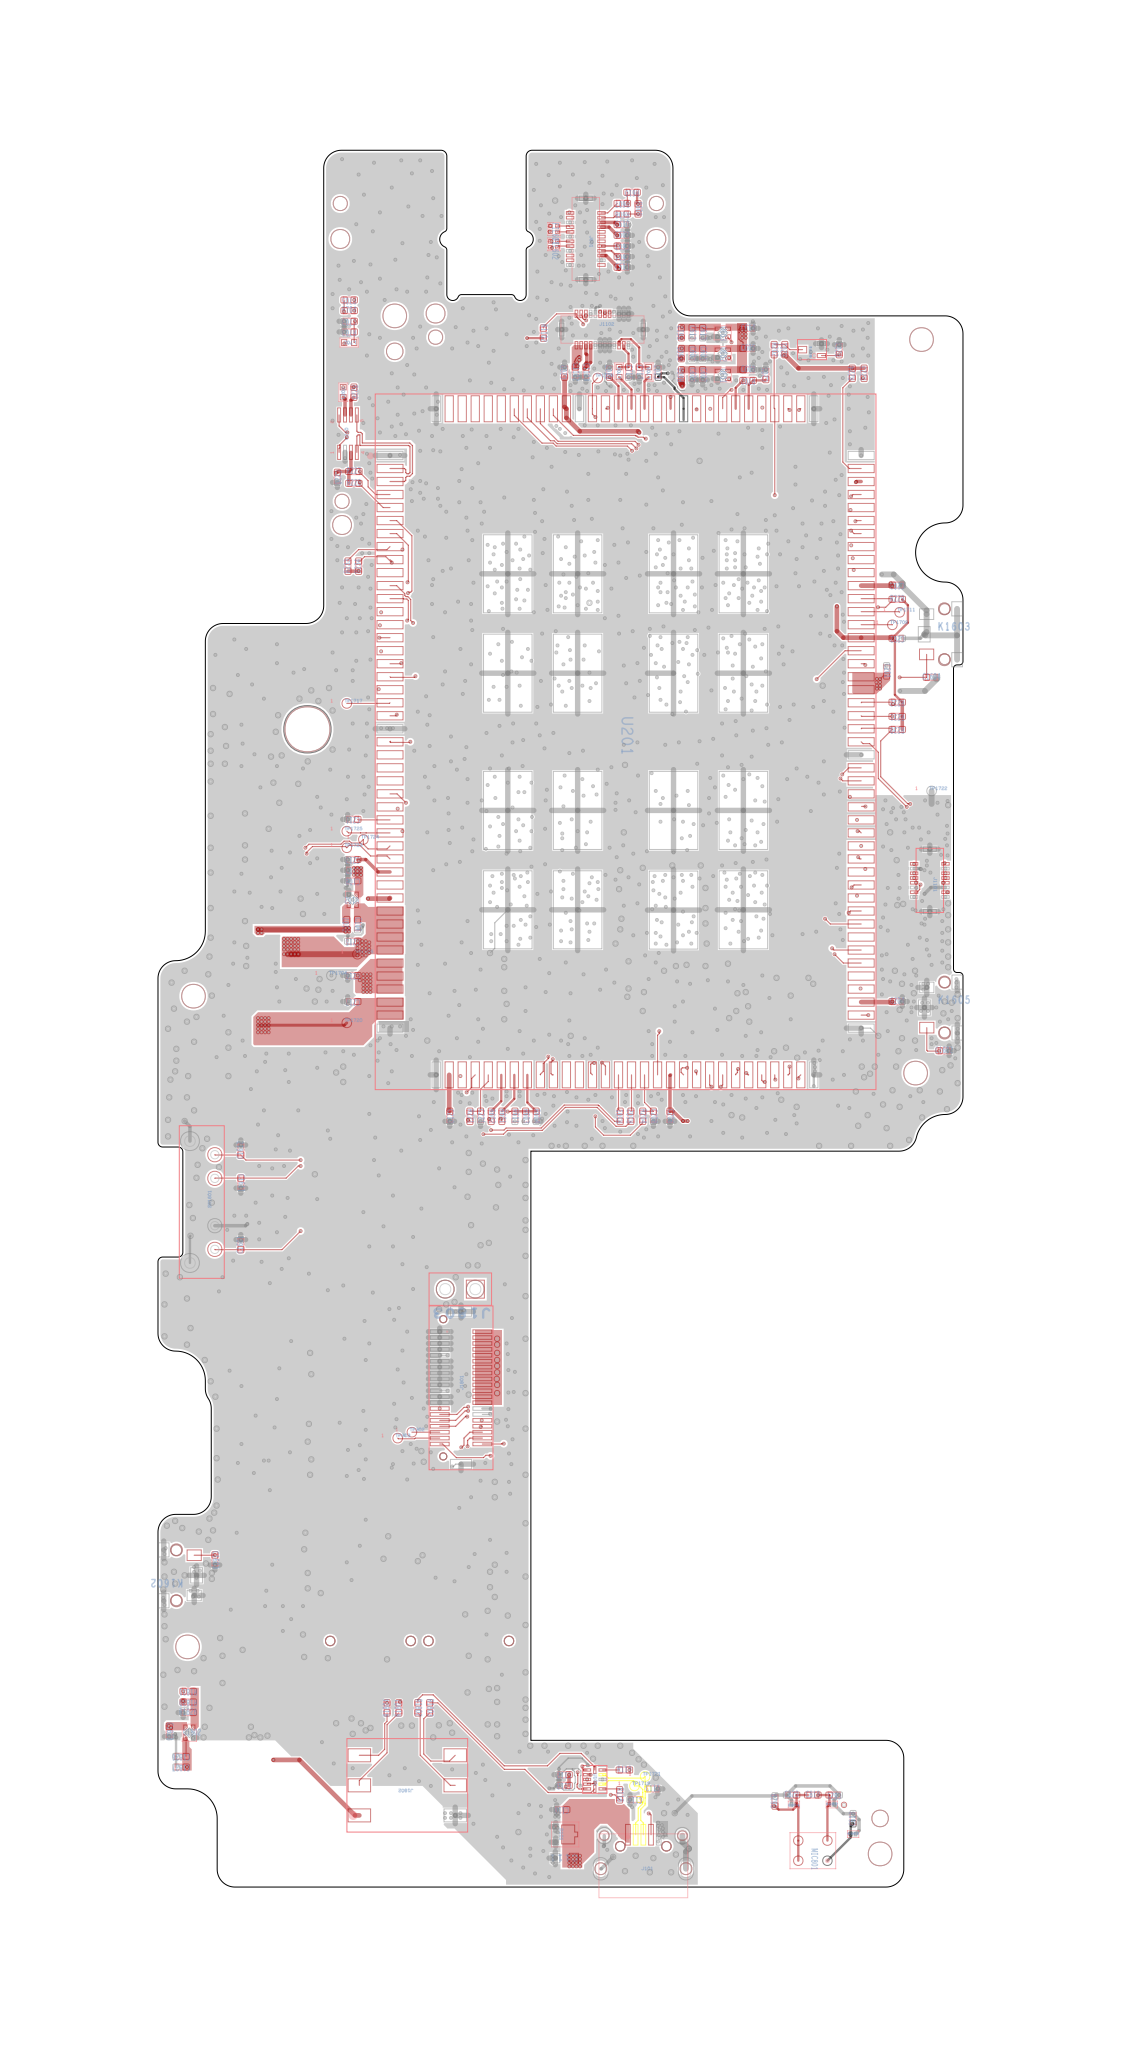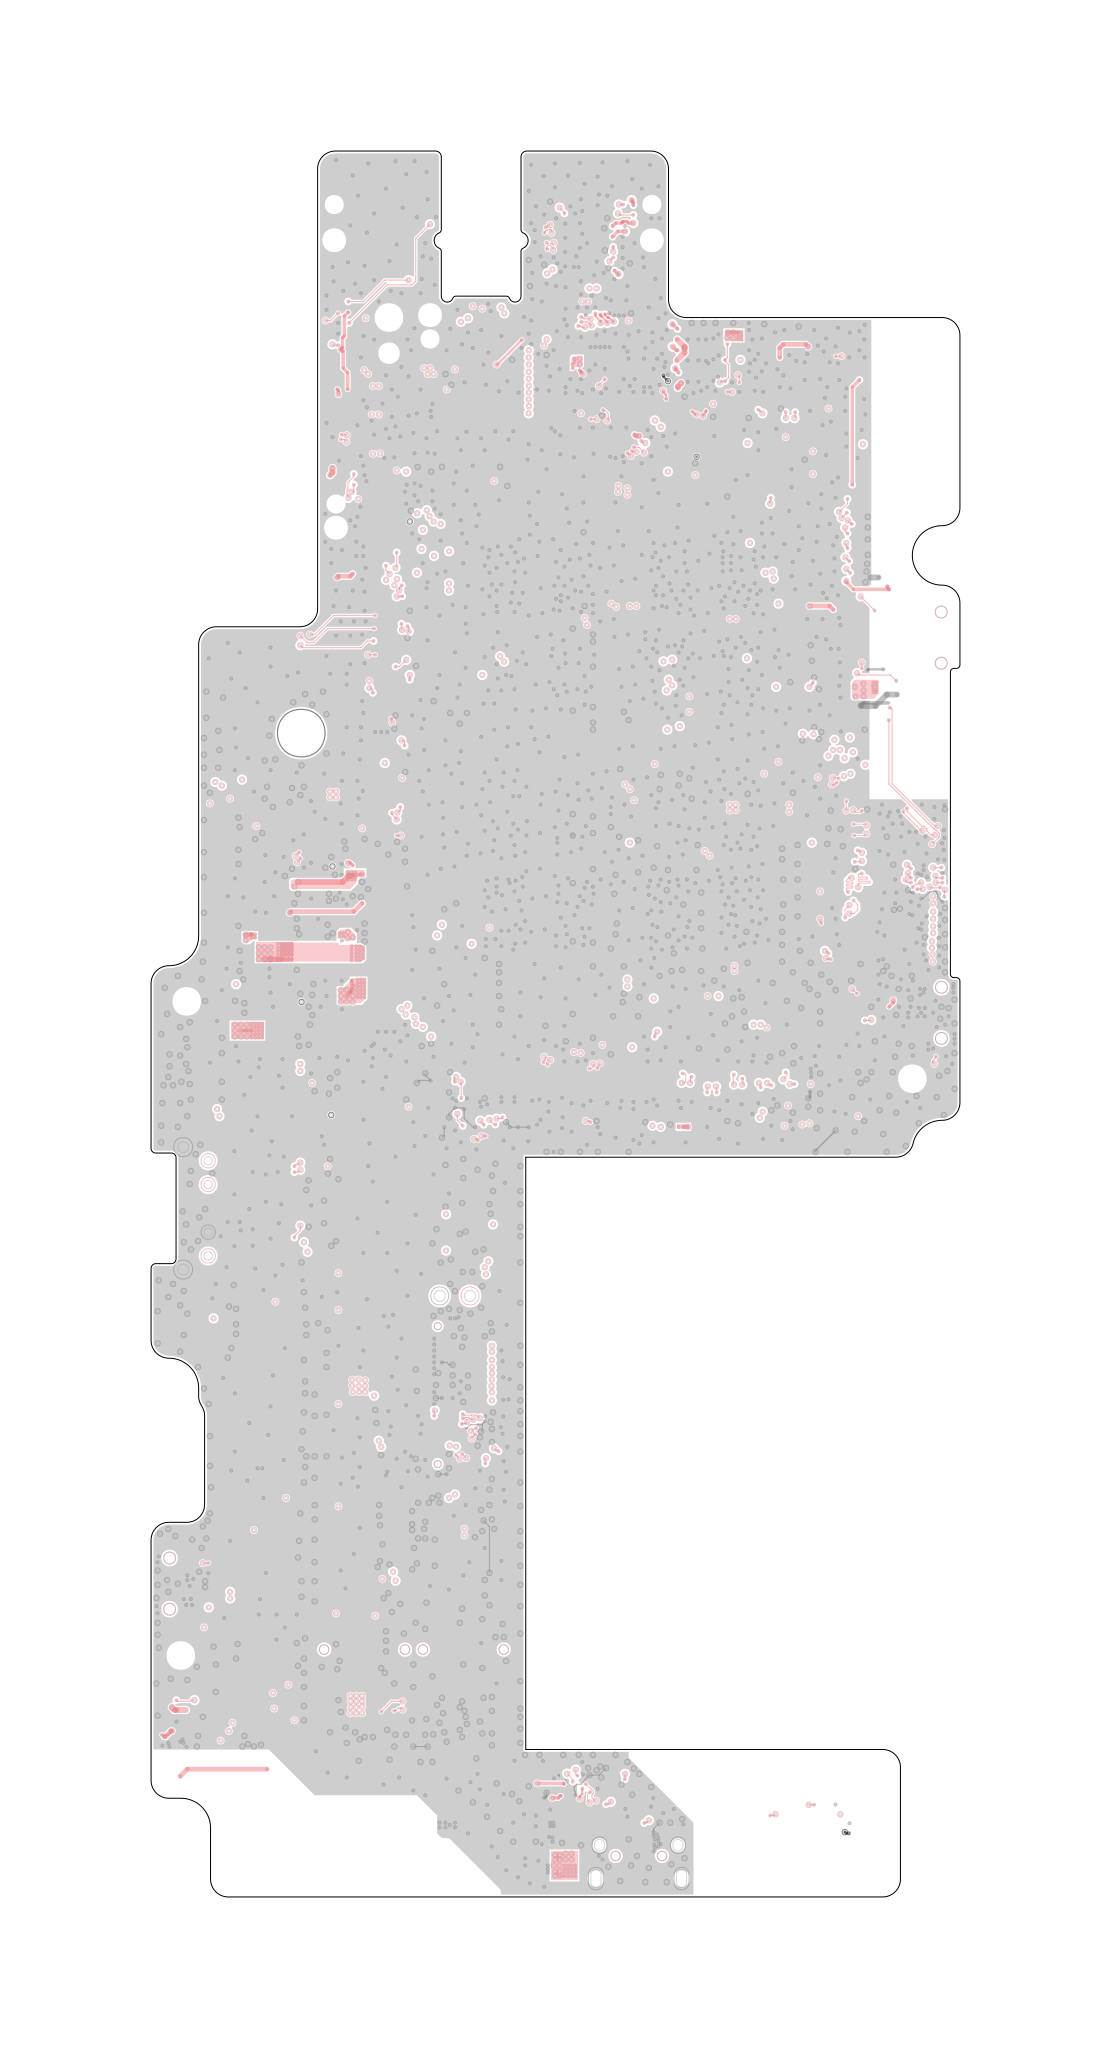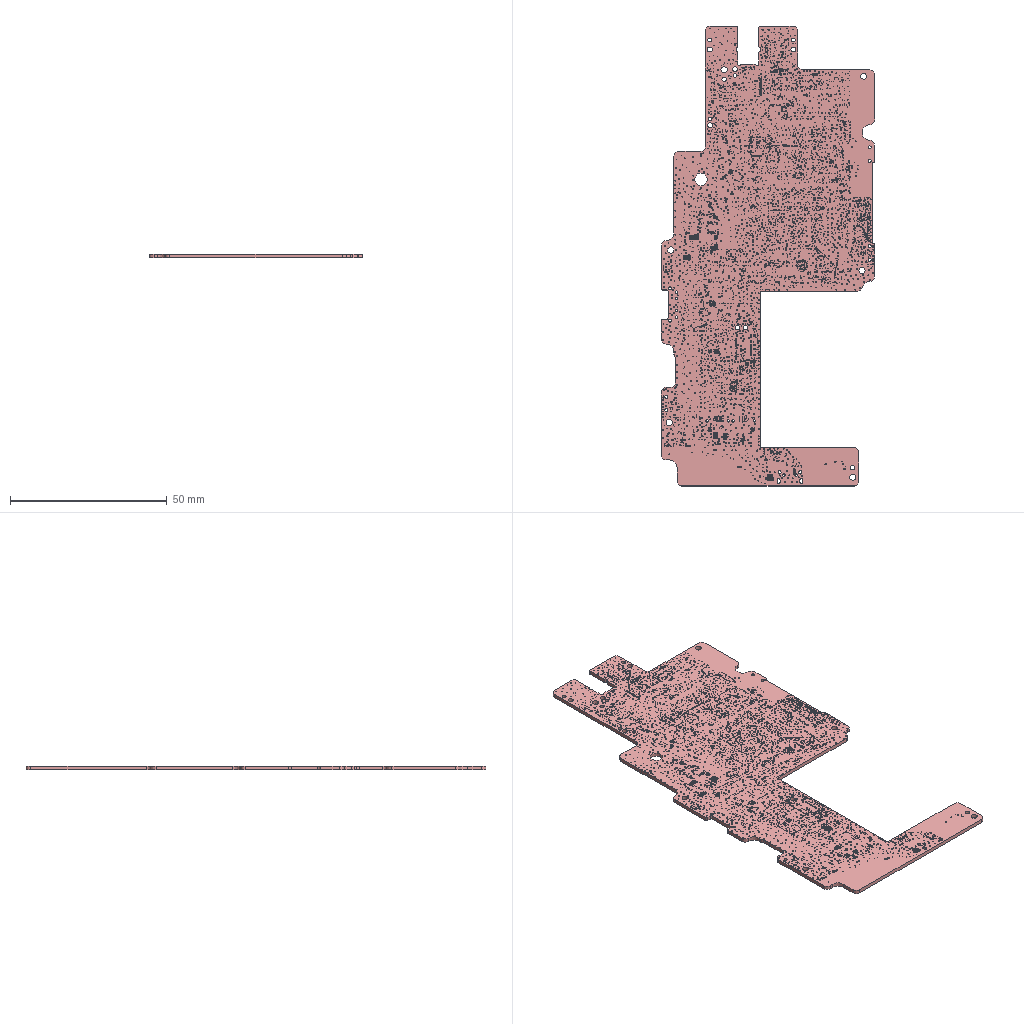Circuit board layout | Cadence Allegro | box 68 x 146.8 x 1.2 mm
Layer stack:
# Cadence Allegro layer stack of  (unit mm; from the constraint file cross-section; dielectric type: 0 not recorded (Allegro does not mark core vs prepreg), 3 surface material)
index,name,kind,layer,copper_thickness_mm,dielectric_type,dielectric_thickness_mm,dielectric_material,dielectric_constant
0,Top Surface,other,,,,,,
1,TOP,copper,TOP,0.0229,,,,
2,Dielectric1,dielectric,,,0,0.381,FR-4,4.5
3,ART02,copper,ART02,0.0178,,,,
4,Dielectric2,dielectric,,,0,0.0889,FR-4,4.5
5,ART03,copper,ART03,0.033,,,,
6,Dielectric3,dielectric,,,0,0.2032,FR-4,4.5
7,ART04,copper,ART04,0.033,,,,
8,Dielectric4,dielectric,,,0,0.0889,FR-4,4.5
9,ART05,copper,ART05,0.0178,,,,
10,Dielectric5,dielectric,,,0,0.381,FR-4,4.5
11,BOTTOM,copper,BOTTOM,0.0229,,,,
12,Bottom Surface,other,,,,,,
# drill layer pairs: low layer,high layer
drill_pair,TOP,BOTTOM
drill_pair,ART05,BOTTOM
Part placement:
REFDES,COMP_VALUE,SYM_NAME,SYM_X,SYM_Y,SYM_ROTATE,SYM_MIRROR
ANT401,BXJ-TH-164-01-W,PAD_ANT_BXJ-TH-164-01-W,147.35,169.01,90.000,YES
ANT402,BXJ-TH-164-01-W,PAD_ANT_BXJ-TH-164-01-W,144.25,169.01,90.000,YES
ANT403,BXJ-TH-164-01-W,PAD_ANT_BXJ-TH-164-01-W,157.89,263.55,180.000,YES
ANT404,BXJ-TH-164-01-W,PAD_ANT_BXJ-TH-164-01-W,157.89,260.45,180.000,YES
ANT405,BXJ-TH-164-01-W,PAD_ANT_BXJ-TH-164-01-W,150.45,169,90.000,YES
ANT406,BXJ-TH-164-01-W,PAD_ANT_BXJ-TH-164-01-W,157.9,266.65,180.000,YES
C101,22U,C0805,118.8,179.8,180.000,YES
C102,10P,C0402,117.9,190.6,270.000,YES
C104,10P,C0402,114.5,190.6,270.000,YES
C105,22U,C0805,113.4,179.8,0.000,YES
C106,1U,C0402,110.9,246.4,270.000,NO
C107,1U,C0402,110.5,251,180.000,NO
C108,10P,C0402,110.5,250.1,180.000,NO
C110,10P,C0402,128.15,171.6,180.000,NO
C111,4.7U,C0603,128.4,167.5,180.000,NO
C112,0.1U,C0402,128.35,174.55,180.000,NO
C113,1U,C0402,128.35,173.65,180.000,NO
C114,10P,C0402,134.35,172.45,180.000,NO
C115,10P,C0402,135.85,173.35,0.000,NO
C201,1U,C0402,155.6,267.85,270.000,NO
C202,1U,C0402,156.5,270.6,180.000,NO
C203,1U,C0402,156.5,275.1,180.000,NO
C204,0.1U,C0402,156.5,239.9,0.000,NO
C205,0.1U,C0402,145.4,292.9,90.000,NO
C206,1U,C0402,137.3,230.2,270.000,NO
C207,0.1U,C0402,136.3,293.1,90.000,NO
C208,10P,C0402,135.9,230.2,270.000,NO
C209,0.1U,C0402,128.4,293.1,90.000,NO
C210,1U,C0402,118.7,230.2,270.000,NO
C211,0.1U,C0402,110.5,255.3,180.000,NO
C213,1U,C0402,110.5,251.9,180.000,NO
C215,2.2U,C0402,110.5,245,180.000,NO
C216,0.1U,C0402,110.5,242.1,180.000,NO
C217,0.1U,C0402,110.5,239.9,180.000,NO
C220,0.1U,C0402,109.2,284.2,270.000,NO
C221,10P,C0402,121.3,230.2,270.000,NO
C224,1U,C0402,146.2,272.5,270.000,YES
C225,10P,C0402,147.1,272.5,270.000,YES
C226,1U,C0402,142.4,272.9,0.000,YES
C227,0.1U,C0402,148.9,272.5,270.000,YES
C301,0.1U,C0402,114.8,223.3,180.000,YES
C302,0.1U,C0402,114.8,228.1,0.000,YES
C303,1U,C0402,106.2,228,90.000,YES
C304,1U,C0402,105,224.7,270.000,YES
C305,0.1U,C0402,105.9,224.7,270.000,YES
C306,1U,C0402,116.1,217.7,0.000,YES
C307,1U,C0402,114,219.65,0.000,YES
C308,10P,C0402,114.45,218.3,90.000,YES
C309,0.1U,C0402,108.9,218.3,90.000,YES
C310,0.1U,C0402,105.9,222.9,90.000,YES
C401,10P,C0402,158.6,289,90.000,YES
C402,0.1U,C0402,124.2,286.7,180.000,YES
C403,470P,C0402,125.7,271.6,90.000,YES
C404,4.7U,C0603,121.9,286.8,0.000,YES
C405,100P,C0402,119.8,272.6,0.000,YES
C406,0.1U,C0402,119.8,271.7,0.000,YES
C407,1U,C0402,112.9,286,90.000,YES
C408,10P,C0402,113.8,286,90.000,YES
C409,1U,C0402,109.5,286,90.000,YES
C410,1U,C0402,110.3,284.6,0.000,YES
C411,0.1U,C0402,119.5,286.7,0.000,YES
C501,1U,C0402,114.4,291.1,90.000,YES
C502,10P,C0402,115.3,291.1,90.000,YES
C503,1U,C0402,110.4,291.6,0.000,YES
C504,1U,C0402,114.4,293,90.000,YES
C505,10P,C0402,115.3,293,90.000,YES
C506,1U,C0402,110.4,293.5,0.000,YES
C507,0.1U,C0402,117.046,261.786,180.000,YES
C508,4.7U,C0402,117.046,262.687,180.000,YES
C509,10U,C0603,114.2,267.7,0.000,YES
C510,10P,C0402,116.1,268.4,270.000,YES
C511,1U,C0402,110.4,289.7,0.000,YES
C512,1U,C0402,115.3,289.2,90.000,YES
C513,10P,C0402,114.4,289.2,90.000,YES
C520,10P,C0402,122.5,298,0.000,YES
C521,10P,C0402,120.7,298,180.000,YES
C522,1U,C0402,117.7,286.7,180.000,YES
C523,10P,C0402,115.9,286.7,0.000,YES
C524,0.1U,C0402,116.2,293,90.000,YES
C525,0.1U,C0402,116.6,290.7,0.000,YES
C526,0.1U,C0402,117.1,289.2,90.000,YES
C601,1U,C0402,140.062,294.669,270.000,NO
C602,10P,C0402,139.162,294.669,270.000,NO
C603,10P,C0402,133.273,303.763,180.000,NO
C604,10P,C0402,133.273,302.863,180.000,NO
C605,1U,C0402,143.9,295.1,0.000,NO
C606,1U,C0402,139.162,292.869,270.000,NO
C607,10P,C0402,140.062,292.869,270.000,NO
C608,1U,C0402,143.9,293.3,0.000,NO
C609,0.1U,C0402,133.273,304.663,0.000,NO
C610,0.1U,C0402,133.273,305.563,0.000,NO
C611,0.1U,C0402,133.273,301.963,0.000,NO
C612,1U,C0402,139.162,296.431,270.000,NO
C613,10P,C0402,140.062,296.431,270.000,NO
C614,1U,C0402,143.9,296.8,0.000,NO
C701,220N,C0402,137.4,268.7,0.000,YES
C702,33P,C0402,109.1,298.8,270.000,YES
C703,33P,C0402,110.2,297.4,180.000,NO
C704,33P,C0402,133.2,296.5,180.000,YES
C705,1U,C0402,133.2,297.4,0.000,YES
C706,33P,C0402,113.5,299.5,180.000,YES
C707,0.1U,C0402,126.7,249.9,0.000,YES
C708,1U,C0402,127.1,255.1,270.000,YES
C709,10P,C0402,128,255.1,270.000,YES
C710,1U,C0402,131.4,255,270.000,YES
C711,22U,C0805,131.2,251.1,90.000,YES
C712,22U,C0805,129.3,251.1,90.000,YES
C713,4.7U,C0402,137.4,269.6,180.000,YES
C714,33P,C0402,134.7,293.1,270.000,NO
C715,33P,C0402,133.8,293.1,270.000,NO
C716,220N,C0402,132,268.2,180.000,YES
C717,0.1U,C0402,128.727,247.493,0.000,YES
C718,22U,C0805,131.135,244.786,270.000,YES
C719,22U,C0805,129.173,244.786,270.000,YES
C801,33N,C0402,140.8,229.4,270.000,YES
C802,0.1U,C0402,128.5,238.2,90.000,YES
C803,0.1U,C0402,139,240.9,180.000,YES
C805,33N,C0402,144.6,230,180.000,YES
C806,33N,C0402,144.6,231.8,0.000,YES
C807,220N,C0402,132.7,232.3,0.000,YES
C808,220N,C0402,129.5,232.8,270.000,YES
C809,220N,C0402,132.7,233.3,0.000,YES
C810,220N,C0402,129.5,234.7,90.000,YES
C811,220N,C0402,132.7,234.2,0.000,YES
C812,220N,C0402,133.2,236.1,270.000,YES
C813,33P,C0402,130.9,236.1,180.000,YES
C814,0.1U,C0402,129.5,237.4,90.000,YES
C817,33N,C0402,137.6,229,0.000,YES
C818,0.1U,C0402,152.77,170.83,90.000,NO
C819,33P,C0402,149.37,172.83,0.000,NO
C820,33P,C0402,147.57,172.83,0.000,NO
C821,33P,C0402,151.17,172.83,180.000,NO
C1001,1U,C0603,151.5,246,0.000,YES
C1002,33P,C0402,153.8,247.7,0.000,YES
C1003,0.1U,C0402,153.8,250.3,0.000,YES
C1004,1U,C0402,154.3,236.1,180.000,YES
C1005,33P,C0402,158,237.8,180.000,YES
C1006,33P,C0402,153.8,246.5,0.000,YES
C1007,33P,C0402,153.8,244.9,0.000,YES
C1008,33P,C0402,152,248.3,0.000,YES
C1009,0.1U,C0402,153.8,248.9,0.000,YES
C1010,0.1U,C0402,155.17,255.04,270.000,YES
C1011,1U,C0402,155.17,253.24,90.000,YES
C1101,33P,C0402,117,272.1,90.000,YES
C1102,0.1U,C0402,129.3,293.1,270.000,NO
C1103,0.1U,C0402,130.2,293.1,270.000,NO
C1104,0.1U,C0402,109.3,277.4,0.000,YES
C1105,33P,C0402,116.1,272.1,270.000,YES
C1106,33P,C0402,113.1,278,0.000,YES
C1107,1U,C0402,100.7,182,0.000,YES
C1201,1UF,C0402,126.5,263.7,90.000,YES
C1202,0.1U,C0402,98,187.3,90.000,YES
C1203,1U,C0402,99.3,187.3,90.000,YES
C1204,0.1U,C0402,101.4,187.3,90.000,YES
C1205,1U,C0402,100.2,187.3,90.000,YES
C1206,0.1U,C0402,136.9,266.9,180.000,YES
C1207,1U,C0402,135.1,266.9,0.000,YES
C1208,0.1U,C0402,132.8,262.8,0.000,YES
C1209,0.1U,C0402,132.8,264.6,0.000,YES
C1501,10P,C0402,111,238.7,270.000,YES
C1502,1U,C0402,116.2,237.4,0.000,YES
C1503,33P,C0402,116.2,238.3,180.000,YES
C1504,10P,C0402,111.9,238.7,270.000,YES
C1505,10P,C0402,114.8,238.7,270.000,YES
C1506,10P,C0402,117.6,238.7,90.000,YES
C1507,10P,C0402,120.4,238.7,270.000,YES
C1508,10P,C0402,121.3,238.7,270.000,YES
C1509,10P,C0402,143.2,258,0.000,YES
C1510,10P,C0402,135.4,258,0.000,YES
C1511,10P,C0402,138,258,0.000,YES
C1512,10P,C0402,140.6,258,0.000,YES
C1513,1U,C0402,140.6,258.9,0.000,YES
C1514,1U,C0402,147.2,258.4,270.000,YES
C1601,10P,C0402,101.049,219.352,90.000,NO
C1602,10P,C0402,160.46,235.74,0.000,NO
C1603,10P,C0402,98.86,192.7,270.000,NO
C1604,10P,C0402,159.39,267.3,0.000,NO
C1605,10P,C0402,100.7,177.9,180.000,YES
C1606,10P,C0402,100.7,178.8,180.000,YES
C1607,10P,C0402,100.7,179.7,180.000,YES
C1608,10P,C0402,105.4,233.8,180.000,YES
C1609,10P,C0402,105.4,234.7,180.000,YES
C1610,10P,C0402,105.4,235.6,180.000,YES
C1611,10P,C0402,101.049,224.552,270.000,NO
C1612,10P,C0402,101.049,227.352,90.000,NO
C1802,22U,C0805,123.7,205.8,90.000,YES
C1803,22U,C0805,123.7,212.2,270.000,YES
C1804,1U,C0402,123.7,210,180.000,YES
C1805,0.1U,C0402,123.7,209,180.000,YES
C1806,0.1U,C0402,123.7,208,180.000,YES
C1812,10U,C0603,115.2,211,270.000,YES
C1813,10U,C0603,115.2,207,90.000,YES
C1814,0.1U,C0402,112.8,199.8,180.000,YES
C1815,0.1U,C0402,121.7,193.5,0.000,YES
C1816,0.1U,C0402,123.1,202.5,180.000,YES
C1817,1U,C0402,117.8,193,0.000,YES
C1818,0.1U,C0402,112.8,198.9,0.000,YES
C1819,0.1U,C0402,121.7,195.3,180.000,YES
C1820,0.1U,C0402,108.4,198.6,180.000,YES
C1821,1U,C0402,110.3,195.5,90.000,YES
C1822,1U,C0402,112.8,198,0.000,YES
C1823,10P,C0402,112.8,197.1,0.000,YES
C1826,10P,C0402,96,176.1,180.000,NO
C1827,1U,C0402,96,175.2,180.000,NO
C1828,1U,C0402,95,178.2,270.000,NO
C1829,10P,C0402,113.5,213.7,180.000,YES
C1830,1U,C0402,113.5,214.6,180.000,YES
C1831,1U,C0402,110.3,215.4,0.000,YES
D101,PTVS12VU1UPA,DFN2020-3,128.45,169.5,270.000,NO
D801,PESD5V0L1BSF,DSN0603-2,147.77,172.03,0.000,NO
D802,PESD5V0L1BSF,DSN0603-2,150.97,172.03,180.000,NO
D803,PESD5V0L1BSF,DSN0603-2,152.77,169.53,180.000,NO
D1001,RB160MM-40,RB160MM-40,151.4,241.6,270.000,YES
D1101,PESD5V0L1BSF,DSN0603-2,112.7,277.2,0.000,YES
D1102,PESD5V0L1BSF,DSN0603-2,110.7,277.2,0.000,YES
D1103,PESD5V0L1BSF,DSN0603-2,111.7,277.2,180.000,YES
D1501,PESD5V0L1BSF,DSN0603-2,117.3,240.6,0.000,YES
D1502,PESD5V0L1BSF,DSN0603-2,116,240.6,0.000,YES
D1504,PESD5V0L1BSF,DSN0603-2,120,240.6,180.000,YES
D1505,PESD5V0L1BSF,DSN0603-2,118.6,240.6,0.000,YES
D1506,PESD5V0L1BSF,DSN0603-2,114.7,240.6,0.000,YES
D1507,PESD5V0L1BSF,DSN0603-2,113.4,240.6,180.000,YES
D1508,PESD5V0L1BSF,DSN0603-2,111.9,240.6,0.000,YES
D1509,PESD5V0L1BSF,DSN0603-2,144.5,258.2,90.000,YES
D1510,PESD5V0L1BSF,DSN0603-2,136.7,258.2,90.000,YES
D1511,PESD5V0L1BSF,DSN0603-2,139.3,258.2,90.000,YES
D1512,PESD5V0L1BSF,DSN0603-2,141.9,258.2,90.000,YES
F401,MGMA5220H2450-A01,MGMA5220H2450-A01,159,283.8,90.000,YES
F405,SAFEB1G57KB0F00,SAFEA1G57KJ0F00,123.45,272.4,180.000,YES
FIL501,ACFT4A2G900E,EMI4_0P85X0P65X0P55_INNOCHIPS,125.15,294.858,90.000,YES
FIL502,ACFT4A2G900E,EMI4_0P85X0P65X0P55_INNOCHIPS,125.15,293.658,90.000,YES
FIL503,ACFT4A2G900E,EMI4_0P85X0P65X0P55_INNOCHIPS,125.15,292.458,90.000,YES
FIL504,ACFT4A2G900E,EMI4_0P85X0P65X0P55_INNOCHIPS,125.15,291.308,90.000,YES
FIL505,ACFT4A2G900E,EMI4_0P85X0P65X0P55_INNOCHIPS,125.15,290.158,90.000,YES
FIL601,ACFT4A2G900E,EMI4_0P85X0P65X0P55_INNOCHIPS,127.5,305.2,270.000,NO
FIL602,ACFT4A2G900E,EMI4_0P85X0P65X0P55_INNOCHIPS,127.5,303.9,270.000,NO
FIL1001,ACFT4A2G900E,EMI4_0P85X0P65X0P55_INNOCHIPS,159.9,245.3,90.000,YES
FIL1002,ACFT4A2G900E,EMI4_0P85X0P65X0P55_INNOCHIPS,159.9,247.7,90.000,YES
FIL1003,ACFT4A2G900E,EMI4_0P85X0P65X0P55_INNOCHIPS,159.9,246.5,90.000,YES
FIL1004,ACFT4A2G900E,EMI4_0P85X0P65X0P55_INNOCHIPS,159.9,248.9,90.000,YES
FIL1005,ACFT4A2G900E,EMI4_0P85X0P65X0P55_INNOCHIPS,159.9,244.1,90.000,YES
J101,U1014-2-DN-W,USB_U1014-2-DN-W,135.05,166.6,0.000,NO
J102,02250370010168,CON_BAT_02250370010168,112.001,186.503,180.000,YES
J103,02250370010168,CON_BAT_02250370010168,120.301,186.503,180.000,YES
J401,20449-001E,ANT_CON_IPEX_20449-001E,128.1,275.7,0.000,YES
J402,20449-001E,ANT_CON_IPEX_20449-001E,128.05,175.52,0.000,YES
J403,20449-001E,ANT_CON_IPEX_20449-001E,159.5,291.8,0.000,YES
J406,20449-001E,ANT_CON_IPEX_20449-001E,157,273.9,0.000,YES
J601,DF37NB-24DS-0_4V,BTB_DF37NB-24DS-0_4V_CW,130.189,304.355,270.000,NO
J701,J303-B06G1-NZL2,JACK_J303-B06G1-NZL2,118.45,311.15,180.000,YES
J1001,DF37NB-24DS-0_4V,BTB_DF37NB-24DS-0_4V_CCW,157.075,246.9,270.000,YES
J1002,DF37NB-10DS-0_4V,BTB_DF37NB-10DS-0_4V_CW,158.07,254.74,270.000,YES
J1101,DF37NB-16DS-0_4V,BTB_DF37NB-16DS-0_4V_CW,159.25,250.14,270.000,NO
J1102,DF37NB-24DS-0_4V,BTB_DF37NB-24DS-0_4V_CW,131.6,296.7,0.000,NO
J1103,DF37NB-16DS-0_4V,BTB_DF37NB-16DS-0_4V_CW,111.4,274.6,0.000,YES
J1501,TF008-015,TF_TF008-015,111.7,251.78,180.000,YES
J1601,DF37NB-10DS-0_4V,BTB_DF37NB-10DS-0_4V_CW,96.1,234.7,90.000,YES
J1602,DF37NB-10DS-0_4V,BTB_DF37NB-10DS-0_4V_CW,97.5,177.6,90.000,YES
J1801,DF12-40DS-0_5V,BTB_DF12-40DS-0_5V_CCW,119.65,207.25,90.000,NO
J1802,ASMFS220A01BR023,CON6_ASMFS220A01BR023,115.11,173.65,180.000,NO
J1803,CON2,SIP2_2_54P,120.86,215.59,180.000,NO
K1602,SKRTLAE010,KEY_SKRTLAE010,95.61,193.55,180.000,NO
K1603,SKRTLAE010,KEY_SKRTLAE010,160.479,268.793,0.000,NO
K1605,SKRTLAE010,KEY_SKRTLAE010,160.495,237.242,0.000,NO
L202,600@100M,L0402,109.7,291.4,90.000,NO
L301,600@100M,L0402,105,222.9,270.000,YES
L302,600@100M,L0402,114.8,229,0.000,YES
L303,600@100M,L0402,116.6,223.3,0.000,YES
L304,600@100M,L0402,108,218.3,270.000,YES
L401,82N,L0402,159.9,289.5,180.000,YES
L402,82N,L0402,159.9,288.5,180.000,YES
L404,82N,L0402,134.5,173.23,270.000,YES
L405,82N,L0402,137.29,173.23,270.000,YES
L406,68N,L0402,126.6,270.7,90.000,YES
L407,82N,L0402,157.4,271.7,180.000,YES
L408,82N,L0402,157.5,269.1,180.000,YES
L501,1U,L2520_VLS252010HBX,114.846,261.687,270.000,YES
L701,2500@100M,L0603,111.1,298.7,0.000,YES
L702,600@100M,L0402,110.2,295.6,180.000,NO
L703,600@100M,L0402,133.2,298.3,180.000,YES
L704,600@100M,L0402,133.2,299.1,0.000,YES
L705,600@100M,L0402,135.5,293.1,90.000,NO
L706,600@100M,L0402,133,293.1,90.000,NO
L707,220@100M,L0603,134.2,272.9,270.000,YES
L708,220@100M,L0603,135.8,272.9,270.000,YES
L801,600@100M,L0402,129.5,239.2,90.000,YES
L802,600@100M,L0402,127.6,239.1,90.000,YES
L803,600@100M,L0402,128.7,240,270.000,YES
L805,600@100M,L0402,132.3,235.6,90.000,YES
L1001,10U,L3030_SPH3012H100MTY01,150.9,237.3,270.000,YES
L1002,600@100M,L0402,152,249.6,180.000,YES
L1802,600@100M,L0402,113.4,206.1,180.000,YES
L1803,600@100M,L0402,123.1,194,270.000,YES
L1804,600@100M,L0402,117.4,206,270.000,YES
MIC801,MSM38A3729H3-C,MSM381A3729H3-C,149.37,168.13,270.000,NO
PAD101,PAD_R1P2X2P2,PAD_R1P2X2P2,130.312,284.215,90.000,YES
PAD102,PAD_R1P2X2P2,PAD_R1P2X2P2,152.412,284.231,90.000,YES
PAD1101,PAD_R1P2X2P2,PAD_R1P5X2P7,103,182,90.000,YES
PAD1102,PAD_R1P2X2P2,PAD_R1P5X2P7,105.5,182,90.000,YES
Q201,WNM4153,SOT-523,149.3,295,90.000,NO
R103,0,R0402,112,190.6,90.000,YES
R104,0,R0402,109.5,190.6,90.000,YES
R106,0,R0402,120.4,190.6,90.000,YES
R107,1K,R0402,110,246.4,90.000,NO
R108,0,R0402,118.8,190.6,90.000,YES
R112,0,R0402,122.7,190.6,90.000,YES
R113,0,R0402,113.6,190.6,90.000,YES
R118,1K,R0402,133.05,172.85,270.000,NO
R119,1K,R0402,133.45,174.95,0.000,NO
R201,10K,R0402,147,295,90.000,NO
R202,1K,R0402,146.1,295,270.000,NO
R203,10K,R0402,151.6,295,90.000,NO
R204,0,R0402,135,230.2,270.000,NO
R220,10K,R0402,110.6,291.4,270.000,NO
R221,0,R0402,120.4,230.2,270.000,NO
R223,10K,R0402,153.7,293,90.000,NO
R224,10K,R0402,152.7,293,90.000,NO
R226,0,R0402,114.3,237.4,180.000,YES
R227,2.2K,R0402,110.6,284.7,0.000,NO
R228,2.2K,R0402,110.6,283.7,0.000,NO
R229,10K,R0402,156.5,273.9,0.000,NO
R230,2.2K,R0402,156.5,262.9,180.000,NO
R231,2.2K,R0402,156.5,264,180.000,NO
R232,10K,R0402,156.5,265.2,180.000,NO
R233,2.2K,R0402,110.1,276.7,90.000,NO
R234,2.2K,R0402,111,276.7,90.000,NO
R235,10K,R0402,142.4,272,180.000,YES
R236,0,R0402,148,272.5,270.000,YES
R237,10K,R0402,150.7,272.5,90.000,YES
R238,10K,R0402,149.8,272.5,90.000,YES
R239,100K,R0402,152.5,270.7,180.000,YES
R240,100K,R0402,152.5,268.9,180.000,YES
R241,100K,R0402,152.5,269.8,180.000,YES
R242,100K,R0402,152.5,268,180.000,YES
R243,100K,R0402,152.5,267.1,180.000,YES
R244,100K,R0402,152.5,266.2,180.000,YES
R245,100K,R0402,150.2,264.4,90.000,YES
R246,100K,R0402,144.1,270.1,180.000,YES
R247,100K,R0402,144.1,269.2,180.000,YES
R248,100K,R0402,144.1,268.3,180.000,YES
R249,100K,R0402,144.1,267.4,180.000,YES
R250,100K,R0402,144.1,266.5,180.000,YES
R251,100K,R0402,146.6,264.4,270.000,YES
R252,100K,R0402,147.5,264.4,270.000,YES
R253,100K,R0402,149.3,264.4,90.000,YES
R254,100K,R0402,148.4,264.4,270.000,YES
R301,0,R0402,111.6,218.3,270.000,YES
R302,0,R0402,110.7,218.3,270.000,YES
R303,0,R0402,112.5,218.3,270.000,YES
R304,0,R0402,109.8,218.3,270.000,YES
R305,0,R0402,114.8,221.8,0.000,YES
R306,0,R0402,107.1,218.3,90.000,YES
R307,0,R0402,106.2,218.3,90.000,YES
R308,0,R0402,107.1,228,270.000,YES
R309,10K,R0402,110.7,228,270.000,YES
R310,10K,R0402,110.7,229.8,270.000,YES
R311,0,R0402,112,228,270.000,YES
R312,10K,R0402,109.8,229.8,270.000,YES
R313,0,R0402,112.9,228,270.000,YES
R314,0,R0402,112.5,229.8,270.000,YES
R315,0,R0402,111.6,229.8,270.000,YES
R316,10K,R0402,118.05,219.1,270.000,YES
R402,0,R0402,157,270.4,90.000,YES
R420,0,R0402,135.9,172.83,180.000,YES
R421,10K,R0402,110.3,283.7,0.000,YES
R422,1K,R0402,112.1,284.6,0.000,YES
R423,1K,R0402,112.1,283.7,0.000,YES
R424,0,R0402,123.9,271,180.000,YES
R425,1K,R0402,125.6,287.1,270.000,YES
R426,1K,R0402,126.6,279.4,90.000,YES
R501,0,R0402,133.1,230.2,90.000,NO
R502,0,R0402,134,230.2,90.000,NO
R503,0,R0402,116.3,295.4,270.000,YES
R504,0,R0402,115.4,295.4,270.000,YES
R505,10K,R0402,110.4,290.6,0.000,YES
R506,0,R0402,110,295.4,90.000,YES
R507,10K,R0402,110.4,292.5,0.000,YES
R508,0,R0402,116.2,289.2,270.000,YES
R509,0,R0402,112.846,265.587,270.000,YES
R510,10K,R0402,110.4,288.7,0.000,YES
R511,0,R0402,119.846,265.587,270.000,YES
R512,10K,R0402,113.746,265.587,90.000,YES
R513,10K,R0402,118.846,265.587,90.000,YES
R514,390K,R0402,119.346,263.286,180.000,YES
R515,470K,R0402,119.346,264.187,180.000,YES
R520,2.2K,R0402,111.8,295.4,270.000,YES
R521,2.2K,R0402,110.9,295.4,270.000,YES
R601,0,R0402,123.1,230.2,270.000,NO
R602,0,R0402,122.2,230.2,270.000,NO
R603,10K,R0402,125.1,230.2,270.000,NO
R604,10K,R0402,126,230.2,270.000,NO
R605,0,R0402,138.262,294.669,90.000,NO
R606,0,R0402,138.262,292.869,90.000,NO
R607,0,R0402,133.273,307.363,180.000,NO
R608,0,R0402,133.273,306.463,180.000,NO
R609,2.2K,R0402,134.6,306.9,270.000,NO
R610,2.2K,R0402,134.1,308.3,180.000,NO
R611,10K,R0402,124.2,230.2,270.000,NO
R612,0,R0402,138.262,296.431,90.000,NO
R701,0,R0402,132,269.1,180.000,YES
R702,2.2K,R0402,143.9,292.4,180.000,NO
R703,1K,R0402,110.2,296.5,180.000,NO
R704,100K,R0402,110.2,298.3,0.000,NO
R705,0,R0402,110.2,299.2,180.000,NO
R706,0,R0402,133.2,295.6,180.000,YES
R707,10K,R0402,132.2,293.1,90.000,NO
R708,10K,R0402,129.7,256.5,0.000,YES
R709,0,R0402,132,270,180.000,YES
R710,100,R0402,139.2,268.7,0.000,YES
R711,100,R0402,132,267.3,0.000,YES
R712,10K,R0402,137.4,270.5,180.000,YES
R713,10K,R0402,127.549,245.537,270.000,YES
R801,0,R0402,137.6,229.9,0.000,YES
R802,1K,R0402,139,229.4,270.000,YES
R803,1K,R0402,139.9,229.4,270.000,YES
R805,0,R0402,144.6,229.1,0.000,YES
R806,1K,R0402,141.7,229.4,270.000,YES
R807,1K,R0402,144.6,232.7,0.000,YES
R808,10K,R0402,130.9,232.3,180.000,YES
R809,1K,R0402,130.9,233.3,0.000,YES
R810,100K,R0402,144.6,233.6,180.000,YES
R811,10K,R0402,130.9,235.2,180.000,YES
R812,0,R0402,144.6,236.1,0.000,YES
R813,1K,R0402,130.9,234.2,0.000,YES
R814,10K,R0402,144.6,235.2,180.000,YES
R815,0,R0402,136.6,240.4,270.000,YES
R816,10K,R0402,139,239.9,0.000,YES
R817,10K,R0402,140.4,240.4,270.000,YES
R818,100K,R0402,137.5,240.4,90.000,YES
R819,0,R0402,141.3,240.4,270.000,YES
R820,0,R0402,144.6,237.1,180.000,YES
R826,0,R0402,144.6,230.9,0.000,YES
R828,0,R0402,135.7,229,0.000,YES
R829,0,R0402,146.17,172.33,90.000,NO
R1001,10K,R0402,158,238.7,180.000,YES
R1002,0,R0402,152,247.1,0.000,YES
R1003,15,R0402,153.8,242.9,0.000,YES
R1004,0,R0402,158,239.6,180.000,YES
R1101,0,R0402,141.9,269.2,0.000,YES
R1102,10K,R0402,126.6,296.4,270.000,NO
R1103,0,R0402,111.3,278,0.000,YES
R1104,0,R0402,141.9,268.3,0.000,YES
R1105,0,R0402,151.1,264.4,90.000,YES
R1106,0,R0402,145.7,264.4,270.000,YES
R1107,0,R0402,144.1,265.6,180.000,YES
R1108,0,R0402,141.9,267.4,180.000,YES
R1109,0,R0402,149.3,262.3,90.000,YES
R1110,0,R0402,147.5,262.3,270.000,YES
R1111,0,R0402,148.4,262.3,90.000,YES
R1112,0,R0402,152.5,265.3,0.000,YES
R1201,0R,R0402,132.8,263.7,0.000,YES
R1202,0R,R0402,97.1,189.2,270.000,YES
R1203,10K,R0402,98,189.2,90.000,YES
R1204,2.2K,R0402,102.3,189.2,270.000,YES
R1205,2.2K,R0402,101.4,189.2,90.000,YES
R1206,10K,R0402,132.8,265.5,180.000,YES
R1207,300R,R0402,123.6,266.4,270.000,YES
R1208,300R,R0402,124.5,266.4,270.000,YES
R1209,0R,R0402,121.7,263.7,270.000,YES
R1211,1.5K,R0402,122.6,263.7,270.000,YES
R1212,1.5K,R0402,127.9,263.7,90.000,YES
R1213,300R,R0402,126.4,265.6,0.000,YES
R1501,0,R0402,119.4,238.7,90.000,YES
R1502,0,R0402,116.2,239.2,180.000,YES
R1503,10K,R0402,110.5,237.4,180.000,YES
R1504,10K,R0402,112.4,237.4,0.000,YES
R1505,10K,R0402,118.5,238.7,90.000,YES
R1506,10K,R0402,119.9,237.4,180.000,YES
R1507,10K,R0402,121.8,237.4,0.000,YES
R1509,0,R0402,122.3,238.7,90.000,YES
R1510,0,R0402,113.8,238.7,90.000,YES
R1511,0,R0402,112.9,238.7,90.000,YES
R1512,0,R0402,110,238.7,90.000,YES
R1513,0,R0402,146.3,258.4,270.000,YES
R1514,10K,R0402,145.4,258.4,270.000,YES
R1515,0,R0402,135.4,258.9,180.000,YES
R1516,0,R0402,138,258.9,180.000,YES
R1517,0,R0402,143.2,258.9,0.000,YES
R1801,0,R0402,114.4,180.2,90.000,NO
R1802,0,R0402,116,180.2,270.000,NO
R1803,0,R0402,117,180.2,270.000,NO
R1804,0,R0402,113.4,180.2,90.000,NO
R1812,0,R0402,108.7,210.1,180.000,YES
R1813,10K,R0402,108.7,209.2,0.000,YES
R1814,100K,R0402,108.7,208.3,0.000,YES
R1815,2.2K,R0402,113.6,212,180.000,YES
R1816,0,R0402,115.3,204.2,180.000,YES
R1817,0,R0402,115.3,203.3,180.000,YES
R1818,10K,R0402,111.7,206.1,180.000,YES
R1819,0,R0402,118.6,206,270.000,YES
R1820,0,R0402,123.1,203.4,180.000,YES
R1821,10K,R0402,123.1,201.6,180.000,YES
R1822,10K,R0402,121.2,197.9,90.000,YES
R1823,10K,R0402,121.7,194.4,180.000,YES
R1824,1K,R0402,108.4,207.1,0.000,YES
R1825,0,R0402,110.2,198.6,180.000,YES
R1826,10K,R0402,111.2,195.5,90.000,YES
R1828,10K,R0402,96.6,179.8,0.000,NO
R1830,1K,R0402,96.6,180.7,180.000,NO
R1831,1K,R0402,96.6,181.6,180.000,NO
R1832,10K,R0402,109.4,214.1,90.000,YES
R1833,1K,R0402,108.5,214.1,270.000,YES
R1834,1K,R0402,107.6,214.1,270.000,YES
SIM1501,C801B06J61ZL2,SIM_C801B06J61ZL2,140.5,255.9,180.000,YES
SW1601,K3-1370D-G2,TOGGLE_SW_K3-1370D-G2,98.851,222.953,90.000,NO
TP201,1 mm,TESTPOINT_32MIL,142.2,270.1,0.000,YES
TP301,1 mm,TESTPOINT_32MIL,119.15,222.5,0.000,YES
TP302,1 mm,TESTPOINT_32MIL,115.5,203.5,0.000,NO
TP303,1 mm,TESTPOINT_32MIL,114.3,203,0.000,NO
TP304,1 mm,TESTPOINT_32MIL,108.6,229.8,270.000,YES
TP305,1 mm,TESTPOINT_32MIL,108.6,228,270.000,YES
TP1701,1 mm,TESTPOINT_32MIL,128.2,233.2,270.000,YES
TP1702,1 mm,TESTPOINT_32MIL,128.2,234.3,270.000,YES
TP1703,1 mm,TESTPOINT_32MIL,125.7,245.2,270.000,YES
TP1704,1 mm,TESTPOINT_32MIL,108.7,242.1,0.000,NO
TP1705,1 mm,TESTPOINT_32MIL,110.9,243.9,0.000,NO
TP1706,1 mm,TESTPOINT_32MIL,131.2,292.6,0.000,NO
TP1707,1 mm,TESTPOINT_32MIL,106.2,229.8,0.000,YES
TP1708,1 mm,TESTPOINT_32MIL,135.1,295.6,0.000,YES
TP1709,1 mm,TESTPOINT_32MIL,156.085,271.74,0.000,NO
TP1711,1 mm,TESTPOINT_32MIL,156.7,272.8,0.000,NO
TP1713,1 mm,TESTPOINT_32MIL,116.2,188.9,0.000,YES
TP1715,1 mm,TESTPOINT_32MIL,116.2,191,0.000,YES
TP1717,1 mm,TESTPOINT_32MIL,110,265.1,0.000,NO
TP1719,1 mm,TESTPOINT_32MIL,134.3,173.6,0.000,NO
TP1720,1 mm,TESTPOINT_32MIL,110,238.1,0.000,NO
TP1721,1 mm,TESTPOINT_32MIL,135.2,174.4,0.000,NO
TP1722,1 mm,TESTPOINT_32MIL,159.4,257.7,0.000,NO
TP1723,1 mm,TESTPOINT_32MIL,110,252.9,0.000,NO
TP1724,1 mm,TESTPOINT_32MIL,111.4,253.6,0.000,NO
TP1725,1 mm,TESTPOINT_32MIL,110,254.3,0.000,NO
TP1726,1 mm,TESTPOINT_32MIL,142.8,260.3,0.000,YES
TP1727,1 mm,TESTPOINT_32MIL,141,260.3,0.000,YES
TP1728,1 mm,TESTPOINT_32MIL,135,260.3,0.000,YES
TP1729,1 mm,TESTPOINT_32MIL,137.6,260.3,0.000,YES
TP1730,1 mm,TESTPOINT_32MIL,147.2,260.3,0.000,YES
U102,NCP114AMX330TCG,UDFN4_1X1X0P7_0P65,110.5,248.5,180.000,NO
U103,TS3USBA225RUTR,UQFN12_2X1P7X0P5_0P4,130.95,174.15,270.000,NO
U201,CC1500,MODULE_CC1500,133.551,261.853,270.000,NO
U203,TCA9539RTWR,QFN24_4X4X0P9_0P5,148.3,268.5,0.000,YES
U204,NCP114AMX180TCG,UDFN4_1X1X0P7_0P65,144.5,272.5,0.000,YES
U210,TXS0102DCUR,SOT-70,110.1,287.9,90.000,NO
U301,NCP114AMX330TCG,UDFN4_1X1X0P7_0P65,116.05,219.15,270.000,YES
U302,TLV320AIC23BIRHDR,QFN28_5X5X0P9_0P5_EP,110.2,223.3,270.000,YES
U401,ST1097B,MODULE_ST1097B,120.2,279.8,270.000,YES
U402,NCP114AMX330TCG,UDFN4_1X1X0P7_0P65,111.2,286.1,90.000,YES
U502,NCP114AMX120TCG,UDFN4_1X1X0P7_0P65,112.6,291.2,90.000,YES
U503,NCP114AMX180TCG,UDFN4_1X1X0P7_0P65,112.6,293.1,90.000,YES
U504,NCP114AMX280TCG,UDFN4_1X1X0P7_0P65,112.6,289.3,90.000,YES
U505,SGM3780,TDFN14_2X3X0P9_0P4,116.246,265.087,0.000,YES
U506,DF37NB-30DS-04V,BTB_DF37NB-30DS-04V_CCW,122.6,292.3,270.000,YES
U601,NCP114AMX280TCG,UDFN4_1X1X0P7_0P65,141.762,292.869,270.000,NO
U602,NCP114AMX180TCG,UDFN4_1X1X0P7_0P65,141.762,294.669,270.000,NO
U603,NCP114AMX180TCG,UDFN4_1X1X0P7_0P65,141.762,296.431,270.000,NO
U701,FSA6157L6X,FSA6157L6X,126.7,248,90.000,YES
U702,NCP114AMX180TCG,UDFN4_1X1X0P7_0P65,129.7,255,270.000,YES
U703,TPA2028D1,TPA2028D1,134.7,269.6,90.000,YES
U704,FSA6157L6X,FSA6157L6X,130.735,247.816,180.000,YES
U802,FM2018NE-380,FM2018NE-380,138.7,235,180.000,YES
U1002,AW9929STR,SOT23_5,154.8,239.3,180.000,YES
U1201,AK09911,BGA8_1P2X1P2X0P5_0P4,99.7,189.4,90.000,YES
U1202,MPU-6500,QFN24_3X3X0P9_0P4_EP,136.5,264.1,270.000,YES
U1203,LP5562TMX_NOPB,DSBGA12_1P218X1P618X0P775_0P4,124.6,263.7,270.000,YES
U1802,NCP114AMX330TCG,UDFN4_1X1X0P7_0P65,96.7,178.1,0.000,NO
U1803,FDC6331L,SSOT6_1P7X3,112.1,209.198,0.000,YES
U1804,TXS0102DCUR,SOT-70,112.6,202.9,270.000,YES
U1805,TXS0102DCUR,SOT-70,119.5,203.4,0.000,YES
U1806,FT232RQ,QFN32_5X5X0P9_0P5,117.4,196.7,90.000,YES
U1807,TS3USB30EDGSR,TS3USB30EDGSR,109,202.887,0.000,YES
U1808,NCP114AMX180TCG,UDFN4_1X1X0P7_0P65,112.8,195.6,90.000,YES
U1809,NCP114AMX330TCG,UDFN4_1X1X0P7_0P65,111.2,213.8,90.000,YES
X301,SG-211SCE-12000,OSC_SG-211SCE-12000,115.1,225.7,90.000,YES
X801,KC2520C-26000,KC2520C,132,238.6,180.000,YES
Pad and via stacks, first 110 of 383 lines:
# Allegro (Cadence) via spans and padstacks; design units: ("millimeters" 4 10000)
# via spans: padstack,start_layer,end_layer,net_example,count
VIA18P10NM,ETCH/TOP,ETCH/BOTTOM,GND,357
VIA01-025-5-B,ETCH/ART05,ETCH/BOTTOM,GND,2424
# Allegro padstack definitions: name,start_layer,end_layer,drill,plating,holeType,type
SMD34X17,"ETCH/TOP","ETCH/TOP",0.0,"NON_PLATED","none","smd"
SMD25X15,"ETCH/TOP","ETCH/TOP",0.0,"PLATED","none","smd"
SMD17X19,"ETCH/TOP","ETCH/TOP",0.0,"PLATED","none","smd"
SMD07X18,"ETCH/TOP","ETCH/TOP",0.0,"PLATED","none","smd"
SMD03X18,"ETCH/TOP","ETCH/TOP",0.0,"PLATED","none","smd"
SMD1X06,"ETCH/TOP","ETCH/TOP",0.0,"PLATED","none","smd"
SMD065X03,"ETCH/TOP","ETCH/TOP",0.0,"PLATED","none","smd"
SQ5,"ETCH/TOP","ETCH/TOP",0.0,"NON_PLATED","none","smd"
PAD13X5,"ETCH/TOP","ETCH/TOP",0.0,"NON_PLATED","none","smd"
PAD13X2,"ETCH/TOP","ETCH/TOP",0.0,"NON_PLATED","none","smd"
PAD41X17,"ETCH/TOP","ETCH/TOP",0.0,"NON_PLATED","none","smd"
SQ24,"ETCH/TOP","ETCH/TOP",0.0,"NON_PLATED","none","smd"
PAD03X09,"ETCH/TOP","ETCH/TOP",0.0,"PLATED","none","smd"
PAD023X05,"ETCH/TOP","ETCH/TOP",0.0,"NON_PLATED","none","smd"
PAD24X165,"ETCH/TOP","ETCH/TOP",0.0,"NON_PLATED","none","smd"
PAD025X1,"ETCH/TOP","ETCH/TOP",0.0,"NON_PLATED","none","smd"
PAD14X08,"ETCH/TOP","ETCH/TOP",0.0,"NON_PLATED","none","smd"
PAD025X08,"ETCH/TOP","ETCH/TOP",0.0,"NON_PLATED","none","smd"
PAD02X08,"ETCH/TOP","ETCH/TOP",0.0,"NON_PLATED","none","smd"
PAD07X12,"ETCH/TOP","ETCH/TOP",0.0,"NON_PLATED","none","smd"
R071X012S,"ETCH/TOP","ETCH/TOP",0.0,"PLATED","none","smd"
CIRCLE035,"ETCH/TOP","ETCH/TOP",0.0,"PLATED","none","smd"
CIRCLE027,"ETCH/TOP","ETCH/TOP",0.0,"NON_PLATED","none","smd"
PAD025X05,"ETCH/TOP","ETCH/TOP",0.0,"NON_PLATED","none","smd"
PAD13X04,"ETCH/TOP","ETCH/TOP",0.0,"NON_PLATED","none","smd"
PAD09X04,"ETCH/TOP","ETCH/TOP",0.0,"NON_PLATED","none","smd"
PAD04X09,"ETCH/TOP","ETCH/TOP",0.0,"NON_PLATED","none","smd"
SQ04,"ETCH/TOP","ETCH/TOP",0.0,"NON_PLATED","none","smd"
PAD02X16,"ETCH/TOP","ETCH/TOP",0.0,"NON_PLATED","none","smd"
PAD2X1,"ETCH/TOP","ETCH/TOP",0.0,"NON_PLATED","none","smd"
PAD025X13,"ETCH/TOP","ETCH/TOP",0.0,"NON_PLATED","none","smd"
PAD18X22,"ETCH/TOP","ETCH/TOP",0.0,"NON_PLATED","none","smd"
PAD04X18,"ETCH/TOP","ETCH/TOP",0.0,"PLATED","none","smd"
PAD21X16,"ETCH/TOP","ETCH/TOP",0.0,"PLATED","none","smd"
SQ19,"ETCH/TOP","ETCH/TOP",0.0,"NON_PLATED","none","smd"
OX0_40Y1_00T,"ETCH/TOP","ETCH/TOP",0.0,"PLATED","none","smd"
PAD20X30,"ETCH/TOP","ETCH/TOP",0.0,"NON_PLATED","none","smd"
PAD08X14,"ETCH/TOP","ETCH/TOP",0.0,"NON_PLATED","none","smd"
PAD04X065,"ETCH/TOP","ETCH/TOP",0.0,"NON_PLATED","none","smd"
PAD12X25,"ETCH/TOP","ETCH/TOP",0.0,"NON_PLATED","none","smd"
PAD18X23,"ETCH/TOP","ETCH/TOP",0.0,"NON_PLATED","none","smd"
PAD18X2,"ETCH/TOP","ETCH/TOP",0.0,"NON_PLATED","none","smd"
PAD1X13,"ETCH/TOP","ETCH/TOP",0.0,"NON_PLATED","none","smd"
PAD12X09,"ETCH/TOP","ETCH/TOP",0.0,"PLATED","none","smd"
PAD09X12,"ETCH/TOP","ETCH/TOP",0.0,"PLATED","none","smd"
PAD08X15,"ETCH/TOP","ETCH/TOP",0.0,"PLATED","none","smd"
PAD18X14,"ETCH/TOP","ETCH/TOP",0.0,"PLATED","none","smd"
PAD13X11,"ETCH/TOP","ETCH/TOP",0.0,"PLATED","none","smd"
PAD14X19,"ETCH/TOP","ETCH/TOP",0.0,"PLATED","none","smd"
PAD1X095,"ETCH/TOP","ETCH/TOP",0.0,"PLATED","none","smd"
SQ18,"ETCH/TOP","ETCH/TOP",0.0,"NON_PLATED","none","smd"
PAD04X08,"ETCH/TOP","ETCH/TOP",0.0,"NON_PLATED","none","smd"
PAD03,"ETCH/TOP","ETCH/TOP",0.0,"NON_PLATED","none","smd"
PAD07X1,"ETCH/TOP","ETCH/TOP",0.0,"NON_PLATED","none","smd"
PAD03X05,"ETCH/TOP","ETCH/TOP",0.0,"NON_PLATED","none","smd"
PAD032X08,"ETCH/TOP","ETCH/TOP",0.0,"NON_PLATED","none","smd"
PAD21,"ETCH/TOP","ETCH/TOP",0.0,"NON_PLATED","none","smd"
PAD22,"ETCH/TOP","ETCH/TOP",0.0,"NON_PLATED","none","smd"
PAD23,"ETCH/TOP","ETCH/TOP",0.0,"NON_PLATED","none","smd"
PAD05X04,"ETCH/TOP","ETCH/TOP",0.0,"NON_PLATED","none","smd"
PAD06X08,"ETCH/TOP","ETCH/TOP",0.0,"NON_PLATED","none","smd"
SMDS60,"ETCH/TOP","ETCH/TOP",0.0,"PLATED","none","smd"
SMD38X34,"ETCH/TOP","ETCH/TOP",0.0,"PLATED","none","smd"
PAD1,"ETCH/TOP","ETCH/TOP",0.0,"NON_PLATED","none","smd"
SMD60X50,"ETCH/TOP","ETCH/TOP",0.0,"PLATED","none","smd"
R065X103S,"ETCH/TOP","ETCH/TOP",0.0,"PLATED","none","smd"
R029X028S,"ETCH/TOP","ETCH/TOP",0.0,"PLATED","none","smd"
R034X015S,"ETCH/TOP","ETCH/TOP",0.0,"PLATED","none","smd"
SH_R063X054S,"ETCH/TOP","ETCH/TOP",0.0,"PLATED","none","smd"
R026X014S,"ETCH/TOP","ETCH/TOP",0.0,"PLATED","none","smd"
R026X021S,"ETCH/TOP","ETCH/TOP",0.0,"PLATED","none","smd"
R036X052S,"ETCH/TOP","ETCH/TOP",0.0,"PLATED","none","smd"
R049X030S,"ETCH/TOP","ETCH/TOP",0.0,"PLATED","none","smd"
C012S,"ETCH/TOP","ETCH/TOP",0.0,"PLATED","none","smd"
R075X055S,"ETCH/TOP","ETCH/TOP",0.0,"PLATED","none","smd"
R012X016S,"ETCH/TOP","ETCH/TOP",0.0,"PLATED","none","smd"
R055X047S,"ETCH/TOP","ETCH/TOP",0.0,"PLATED","none","smd"
R018X020S,"ETCH/TOP","ETCH/TOP",0.0,"PLATED","none","smd"
R060X080S,"ETCH/TOP","ETCH/TOP",0.0,"PLATED","none","smd"
R070X112S,"ETCH/TOP","ETCH/TOP",0.0,"PLATED","none","smd"
R050X040S,"ETCH/TOP","ETCH/TOP",0.0,"PLATED","none","smd"
R051X059S,"ETCH/TOP","ETCH/TOP",0.0,"PLATED","none","smd"
R039X032S,"ETCH/TOP","ETCH/TOP",0.0,"PLATED","none","smd"
R016X024S,"ETCH/TOP","ETCH/TOP",0.0,"PLATED","none","smd"
O035X060S,"ETCH/TOP","ETCH/TOP",0.0,"PLATED","none","smd"
O035X045S,"ETCH/TOP","ETCH/TOP",0.0,"PLATED","none","smd"
C025S,"ETCH/TOP","ETCH/TOP",0.0,"PLATED","none","smd"
C039SXP,"ETCH/TOP","ETCH/TOP",0.0,"PLATED","none","smd"
R039X027S,"ETCH/TOP","ETCH/TOP",0.0,"PLATED","none","smd"
C015S,"ETCH/TOP","ETCH/TOP",0.0,"PLATED","none","smd"
S103SXP,"ETCH/TOP","ETCH/TOP",0.0,"PLATED","none","smd"
O028X011S,"ETCH/TOP","ETCH/TOP",0.0,"PLATED","none","smd"
O011X028S,"ETCH/TOP","ETCH/TOP",0.0,"PLATED","none","smd"
R016X050S,"ETCH/TOP","ETCH/TOP",0.0,"PLATED","none","smd"
R051X018S,"ETCH/TOP","ETCH/TOP",0.0,"PLATED","none","smd"
R012X025S,"ETCH/TOP","ETCH/TOP",0.0,"PLATED","none","smd"
R063X016S,"ETCH/TOP","ETCH/TOP",0.0,"PLATED","none","smd"
R019X012S,"ETCH/TOP","ETCH/TOP",0.0,"PLATED","none","smd"
R021X012S,"ETCH/TOP","ETCH/TOP",0.0,"PLATED","none","smd"
S136SXP,"ETCH/TOP","ETCH/TOP",0.0,"PLATED","none","smd"
R028X011S,"ETCH/TOP","ETCH/TOP",0.0,"PLATED","none","smd"
C010S,"ETCH/TOP","ETCH/TOP",0.0,"PLATED","none","smd"
R017X011S,"ETCH/TOP","ETCH/TOP",0.0,"PLATED","none","smd"
PAD1X28,"ETCH/TOP","ETCH/TOP",0.0,"NON_PLATED","none","smd"
SMD13X25,"ETCH/TOP","ETCH/TOP",0.0,"NON_PLATED","none","smd"
Design rules, without the lines most boards share, first 8 of 928 lines:
# Cadence Allegro design rules of  (from the Constraint Manager export constraints.dcfx, design unit mm; typed fields in mm)
# columns: name | kind | enabled | priority | scope1 | scope2 | descriptor | typed fields (field=value)
# Allegro precedence (priority 1 wins): 1 Region class-to-class, 2 Region class, 3 Region, 4 class-to-class, 5 DiffPair/Bus/NetGroup override, 6 NetClass, 7 constraint set (CSet) default
# per-layer values are written LAYER=value in the descriptor and LAYER:mm in the typed field; a maximum of 0 means no limit set
# --- net classes (and buses / net groups) ---
NET_VCORE | NetClass | enabled | 6 | no members | All | Net Class (members: 0) |
NET_VCOREDIG | NetClass | enabled | 6 | no members | All | Net Class (members: 0) |
NET_3VANA_PMIC | NetClass | enabled | 6 | no members | All | Net Class (members: 0) |